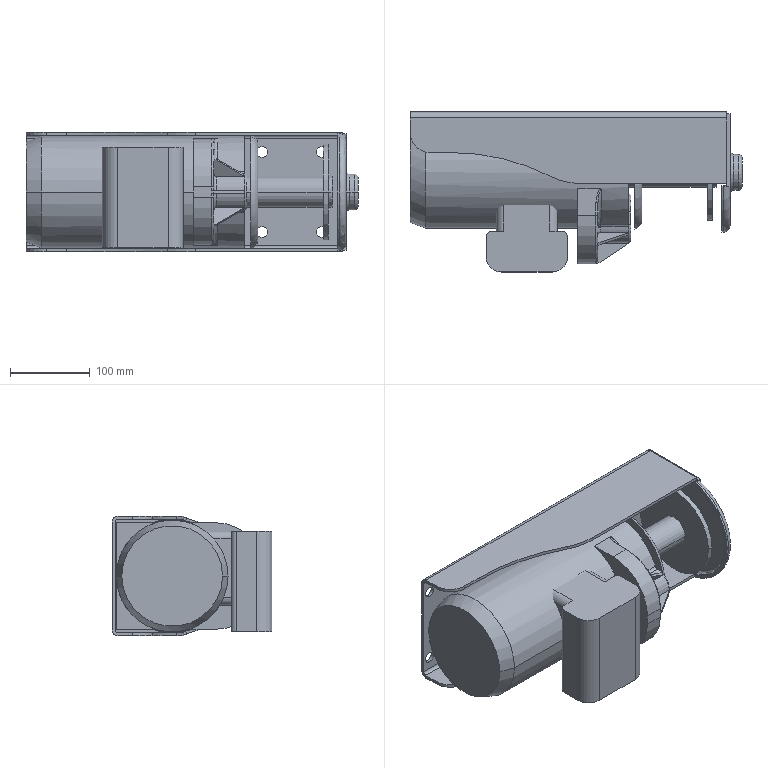Part | STEP file | Pittsburgh Hoist^Pittsburgh Automotive 1300lb remote controlled electric hoist - Representation | 7 solids | 162 faces | box 415.037 x 200.01 x 149.835 mm | volume 6132353 mm3 | plane 81 | cylinder 55 | torus 14 | cone 6 | spline 6 | commonest cylinder face diameters 13.492 x12 38.1 x6 139.7 x6 46.99 x5 19.05 x4 120.65 x4